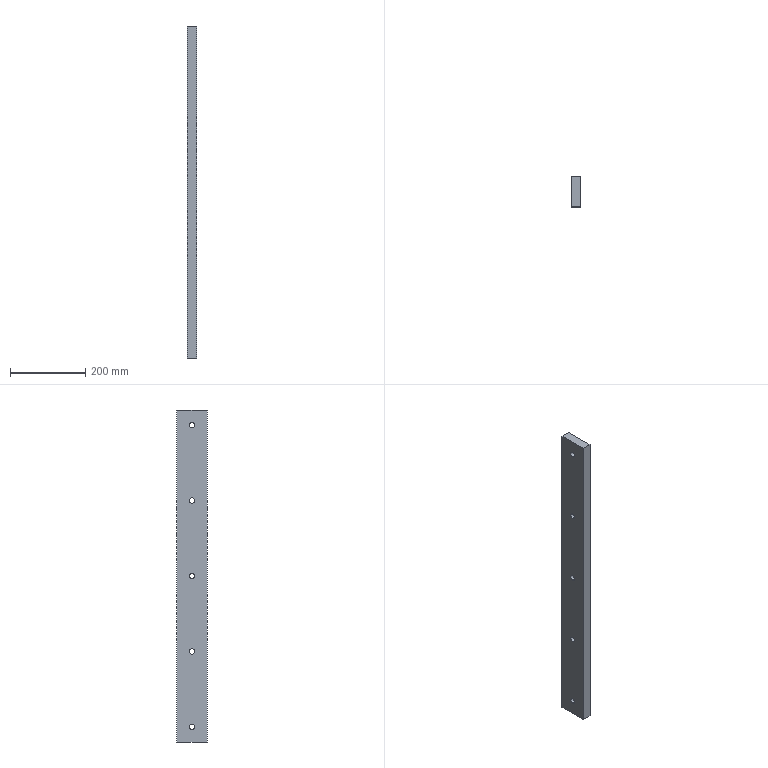Part | SolidWorks | features BaseBody 1 | 1 solid | 16 faces | box 25 x 80 x 880 mm | volume 1740758 mm3 | cylinder 10 | plane 6 | commonest cylinder face diameters 14 x10
STEP:
#1=CARTESIAN_POINT('',(-12.5,0.,407.));
#2=VERTEX_POINT('',#1);
#3=CARTESIAN_POINT('',(-12.5,0.,393.));
#4=VERTEX_POINT('',#3);
#5=CARTESIAN_POINT('',(-12.5,0.,400.));
#6=DIRECTION('',(1.,0.,0.));
#7=DIRECTION('',(0.,0.,-1.));
#8=AXIS2_PLACEMENT_3D('',#5,#6,#7);
#9=CIRCLE('',#8,7.);
#10=EDGE_CURVE('',#2,#4,#9,.T.);
#11=ORIENTED_EDGE('',*,*,#10,.F.);
#12=CARTESIAN_POINT('',(12.5,0.,407.));
#13=VERTEX_POINT('',#12);
#14=CARTESIAN_POINT('',(12.5,0.,407.));
#15=DIRECTION('',(1.,0.,0.));
#16=VECTOR('',#15,1000.);
#17=LINE('',#14,#16);
#18=EDGE_CURVE('',#2,#13,#17,.T.);
#19=ORIENTED_EDGE('',*,*,#18,.T.);
#20=CARTESIAN_POINT('',(12.5,0.,393.));
#21=VERTEX_POINT('',#20);
#22=CARTESIAN_POINT('',(12.5,0.,400.));
#23=DIRECTION('',(1.,0.,0.));
#24=DIRECTION('',(0.,0.,-1.));
#25=AXIS2_PLACEMENT_3D('',#22,#23,#24);
#26=CIRCLE('',#25,7.);
#27=EDGE_CURVE('',#13,#21,#26,.T.);
#28=ORIENTED_EDGE('',*,*,#27,.T.);
#29=CARTESIAN_POINT('',(12.5,0.,393.));
#30=DIRECTION('',(1.,0.,0.));
#31=VECTOR('',#30,1000.);
#32=LINE('',#29,#31);
#33=EDGE_CURVE('',#4,#21,#32,.T.);
#34=ORIENTED_EDGE('',*,*,#33,.F.);
#35=EDGE_LOOP('',(#11,#19,#28,#34));
#36=FACE_OUTER_BOUND('',#35,.T.);
#37=CARTESIAN_POINT('',(12.5,0.,400.));
#38=DIRECTION('',(1.,0.,0.));
#39=DIRECTION('',(0.,0.,-1.));
#40=AXIS2_PLACEMENT_3D('',#37,#38,#39);
#41=CYLINDRICAL_SURFACE('',#40,7.);
#42=ADVANCED_FACE('',(#36),#41,.F.);
#43=CARTESIAN_POINT('',(-12.5,0.,207.));
#44=VERTEX_POINT('',#43);
#45=CARTESIAN_POINT('',(-12.5,0.,193.));
#46=VERTEX_POINT('',#45);
#47=CARTESIAN_POINT('',(-12.5,0.,200.));
#48=DIRECTION('',(1.,0.,0.));
#49=DIRECTION('',(0.,0.,-1.));
#50=AXIS2_PLACEMENT_3D('',#47,#48,#49);
#51=CIRCLE('',#50,7.);
#52=EDGE_CURVE('',#44,#46,#51,.T.);
#53=ORIENTED_EDGE('',*,*,#52,.F.);
#54=CARTESIAN_POINT('',(12.5,0.,207.));
#55=VERTEX_POINT('',#54);
#56=CARTESIAN_POINT('',(12.5,0.,207.));
#57=DIRECTION('',(1.,0.,0.));
#58=VECTOR('',#57,1000.);
#59=LINE('',#56,#58);
#60=EDGE_CURVE('',#44,#55,#59,.T.);
#61=ORIENTED_EDGE('',*,*,#60,.T.);
#62=CARTESIAN_POINT('',(12.5,0.,193.));
#63=VERTEX_POINT('',#62);
#64=CARTESIAN_POINT('',(12.5,0.,200.));
#65=DIRECTION('',(1.,0.,0.));
#66=DIRECTION('',(0.,0.,-1.));
#67=AXIS2_PLACEMENT_3D('',#64,#65,#66);
#68=CIRCLE('',#67,7.);
#69=EDGE_CURVE('',#55,#63,#68,.T.);
#70=ORIENTED_EDGE('',*,*,#69,.T.);
#71=CARTESIAN_POINT('',(12.5,0.,193.));
#72=DIRECTION('',(1.,0.,0.));
#73=VECTOR('',#72,1000.);
#74=LINE('',#71,#73);
#75=EDGE_CURVE('',#46,#63,#74,.T.);
#76=ORIENTED_EDGE('',*,*,#75,.F.);
#77=EDGE_LOOP('',(#53,#61,#70,#76));
#78=FACE_OUTER_BOUND('',#77,.T.);
#79=CARTESIAN_POINT('',(12.5,0.,200.));
#80=DIRECTION('',(1.,0.,0.));
#81=DIRECTION('',(0.,0.,-1.));
#82=AXIS2_PLACEMENT_3D('',#79,#80,#81);
#83=CYLINDRICAL_SURFACE('',#82,7.);
#84=ADVANCED_FACE('',(#78),#83,.F.);
#85=CARTESIAN_POINT('',(-12.5,0.,7.));
#86=VERTEX_POINT('',#85);
#87=CARTESIAN_POINT('',(-12.5,0.,-7.));
#88=VERTEX_POINT('',#87);
#89=CARTESIAN_POINT('',(-12.5,0.,0.));
#90=DIRECTION('',(1.,0.,0.));
#91=DIRECTION('',(0.,0.,-1.));
#92=AXIS2_PLACEMENT_3D('',#89,#90,#91);
#93=CIRCLE('',#92,7.);
#94=EDGE_CURVE('',#86,#88,#93,.T.);
#95=ORIENTED_EDGE('',*,*,#94,.F.);
#96=CARTESIAN_POINT('',(12.5,0.,7.));
#97=VERTEX_POINT('',#96);
#98=CARTESIAN_POINT('',(12.5,0.,7.));
#99=DIRECTION('',(1.,0.,0.));
#100=VECTOR('',#99,1000.);
#101=LINE('',#98,#100);
#102=EDGE_CURVE('',#86,#97,#101,.T.);
#103=ORIENTED_EDGE('',*,*,#102,.T.);
#104=CARTESIAN_POINT('',(12.5,0.,-7.));
#105=VERTEX_POINT('',#104);
#106=CARTESIAN_POINT('',(12.5,0.,0.));
#107=DIRECTION('',(1.,0.,0.));
#108=DIRECTION('',(0.,0.,-1.));
#109=AXIS2_PLACEMENT_3D('',#106,#107,#108);
#110=CIRCLE('',#109,7.);
#111=EDGE_CURVE('',#97,#105,#110,.T.);
#112=ORIENTED_EDGE('',*,*,#111,.T.);
#113=CARTESIAN_POINT('',(12.5,0.,-7.));
#114=DIRECTION('',(1.,0.,0.));
#115=VECTOR('',#114,1000.);
#116=LINE('',#113,#115);
#117=EDGE_CURVE('',#88,#105,#116,.T.);
#118=ORIENTED_EDGE('',*,*,#117,.F.);
#119=EDGE_LOOP('',(#95,#103,#112,#118));
#120=FACE_OUTER_BOUND('',#119,.T.);
#121=CARTESIAN_POINT('',(12.5,0.,0.));
#122=DIRECTION('',(1.,0.,0.));
#123=DIRECTION('',(0.,0.,-1.));
#124=AXIS2_PLACEMENT_3D('',#121,#122,#123);
#125=CYLINDRICAL_SURFACE('',#124,7.);
#126=ADVANCED_FACE('',(#120),#125,.F.);
#127=CARTESIAN_POINT('',(-12.5,0.,-193.));
#128=VERTEX_POINT('',#127);
#129=CARTESIAN_POINT('',(-12.5,0.,-207.));
#130=VERTEX_POINT('',#129);
#131=CARTESIAN_POINT('',(-12.5,0.,-200.));
#132=DIRECTION('',(1.,0.,0.));
#133=DIRECTION('',(0.,0.,-1.));
#134=AXIS2_PLACEMENT_3D('',#131,#132,#133);
#135=CIRCLE('',#134,7.);
#136=EDGE_CURVE('',#128,#130,#135,.T.);
#137=ORIENTED_EDGE('',*,*,#136,.F.);
#138=CARTESIAN_POINT('',(12.5,0.,-193.));
#139=VERTEX_POINT('',#138);
#140=CARTESIAN_POINT('',(12.5,0.,-193.));
#141=DIRECTION('',(1.,0.,0.));
#142=VECTOR('',#141,1000.);
#143=LINE('',#140,#142);
#144=EDGE_CURVE('',#128,#139,#143,.T.);
#145=ORIENTED_EDGE('',*,*,#144,.T.);
#146=CARTESIAN_POINT('',(12.5,0.,-207.));
#147=VERTEX_POINT('',#146);
#148=CARTESIAN_POINT('',(12.5,0.,-200.));
#149=DIRECTION('',(1.,0.,0.));
#150=DIRECTION('',(0.,0.,-1.));
#151=AXIS2_PLACEMENT_3D('',#148,#149,#150);
#152=CIRCLE('',#151,7.);
#153=EDGE_CURVE('',#139,#147,#152,.T.);
#154=ORIENTED_EDGE('',*,*,#153,.T.);
#155=CARTESIAN_POINT('',(12.5,0.,-207.));
#156=DIRECTION('',(1.,0.,0.));
#157=VECTOR('',#156,1000.);
#158=LINE('',#155,#157);
#159=EDGE_CURVE('',#130,#147,#158,.T.);
#160=ORIENTED_EDGE('',*,*,#159,.F.);
#161=EDGE_LOOP('',(#137,#145,#154,#160));
#162=FACE_OUTER_BOUND('',#161,.T.);
#163=CARTESIAN_POINT('',(12.5,0.,-200.));
#164=DIRECTION('',(1.,0.,0.));
#165=DIRECTION('',(0.,0.,-1.));
#166=AXIS2_PLACEMENT_3D('',#163,#164,#165);
#167=CYLINDRICAL_SURFACE('',#166,7.);
#168=ADVANCED_FACE('',(#162),#167,.F.);
#169=CARTESIAN_POINT('',(-12.5,0.,-393.));
#170=VERTEX_POINT('',#169);
#171=CARTESIAN_POINT('',(-12.5,0.,-407.));
#172=VERTEX_POINT('',#171);
#173=CARTESIAN_POINT('',(-12.5,0.,-400.));
#174=DIRECTION('',(1.,0.,0.));
#175=DIRECTION('',(0.,0.,-1.));
#176=AXIS2_PLACEMENT_3D('',#173,#174,#175);
#177=CIRCLE('',#176,7.);
#178=EDGE_CURVE('',#170,#172,#177,.T.);
#179=ORIENTED_EDGE('',*,*,#178,.F.);
#180=CARTESIAN_POINT('',(12.5,0.,-393.));
#181=VERTEX_POINT('',#180);
#182=CARTESIAN_POINT('',(12.5,0.,-393.));
#183=DIRECTION('',(1.,0.,0.));
#184=VECTOR('',#183,1000.);
#185=LINE('',#182,#184);
#186=EDGE_CURVE('',#170,#181,#185,.T.);
#187=ORIENTED_EDGE('',*,*,#186,.T.);
#188=CARTESIAN_POINT('',(12.5,0.,-407.));
#189=VERTEX_POINT('',#188);
#190=CARTESIAN_POINT('',(12.5,0.,-400.));
#191=DIRECTION('',(1.,0.,0.));
#192=DIRECTION('',(0.,0.,-1.));
#193=AXIS2_PLACEMENT_3D('',#190,#191,#192);
#194=CIRCLE('',#193,7.);
#195=EDGE_CURVE('',#181,#189,#194,.T.);
#196=ORIENTED_EDGE('',*,*,#195,.T.);
#197=CARTESIAN_POINT('',(12.5,0.,-407.));
#198=DIRECTION('',(1.,0.,0.));
#199=VECTOR('',#198,1000.);
#200=LINE('',#197,#199);
#201=EDGE_CURVE('',#172,#189,#200,.T.);
#202=ORIENTED_EDGE('',*,*,#201,.F.);
#203=EDGE_LOOP('',(#179,#187,#196,#202));
#204=FACE_OUTER_BOUND('',#203,.T.);
#205=CARTESIAN_POINT('',(12.5,0.,-400.));
#206=DIRECTION('',(1.,0.,0.));
#207=DIRECTION('',(0.,0.,-1.));
#208=AXIS2_PLACEMENT_3D('',#205,#206,#207);
#209=CYLINDRICAL_SURFACE('',#208,7.);
#210=ADVANCED_FACE('',(#204),#209,.F.);
#211=CARTESIAN_POINT('',(-12.5,-40.,-440.));
#212=VERTEX_POINT('',#211);
#213=CARTESIAN_POINT('',(-12.5,40.,-440.));
#214=VERTEX_POINT('',#213);
#215=CARTESIAN_POINT('',(-12.5,40.,-440.));
#216=DIRECTION('',(0.,1.,0.));
#217=VECTOR('',#216,1000.);
#218=LINE('',#215,#217);
#219=EDGE_CURVE('',#212,#214,#218,.T.);
#220=ORIENTED_EDGE('',*,*,#219,.T.);
#221=CARTESIAN_POINT('',(12.5,40.,-440.));
#222=VERTEX_POINT('',#221);
#223=CARTESIAN_POINT('',(12.5,40.,-440.));
#224=DIRECTION('',(-1.,0.,0.));
#225=VECTOR('',#224,1000.);
#226=LINE('',#223,#225);
#227=EDGE_CURVE('',#222,#214,#226,.T.);
#228=ORIENTED_EDGE('',*,*,#227,.F.);
#229=CARTESIAN_POINT('',(12.5,-40.,-440.));
#230=VERTEX_POINT('',#229);
#231=CARTESIAN_POINT('',(12.5,40.,-440.));
#232=DIRECTION('',(0.,1.,0.));
#233=VECTOR('',#232,1000.);
#234=LINE('',#231,#233);
#235=EDGE_CURVE('',#230,#222,#234,.T.);
#236=ORIENTED_EDGE('',*,*,#235,.F.);
#237=CARTESIAN_POINT('',(12.5,-40.,-440.));
#238=DIRECTION('',(-1.,0.,0.));
#239=VECTOR('',#238,1000.);
#240=LINE('',#237,#239);
#241=EDGE_CURVE('',#230,#212,#240,.T.);
#242=ORIENTED_EDGE('',*,*,#241,.T.);
#243=EDGE_LOOP('',(#220,#228,#236,#242));
#244=FACE_OUTER_BOUND('',#243,.T.);
#245=CARTESIAN_POINT('',(12.5,40.,-440.));
#246=DIRECTION('',(0.,0.,1.));
#247=DIRECTION('',(1.,0.,0.));
#248=AXIS2_PLACEMENT_3D('',#245,#246,#247);
#249=PLANE('',#248);
#250=ADVANCED_FACE('',(#244),#249,.F.);
#251=CARTESIAN_POINT('',(-12.5,40.,440.));
#252=VERTEX_POINT('',#251);
#253=CARTESIAN_POINT('',(-12.5,40.,440.));
#254=DIRECTION('',(0.,0.,1.));
#255=VECTOR('',#254,1000.);
#256=LINE('',#253,#255);
#257=EDGE_CURVE('',#214,#252,#256,.T.);
#258=ORIENTED_EDGE('',*,*,#257,.T.);
#259=CARTESIAN_POINT('',(12.5,40.,440.));
#260=VERTEX_POINT('',#259);
#261=CARTESIAN_POINT('',(12.5,40.,440.));
#262=DIRECTION('',(-1.,0.,0.));
#263=VECTOR('',#262,1000.);
#264=LINE('',#261,#263);
#265=EDGE_CURVE('',#260,#252,#264,.T.);
#266=ORIENTED_EDGE('',*,*,#265,.F.);
#267=CARTESIAN_POINT('',(12.5,40.,440.));
#268=DIRECTION('',(0.,0.,1.));
#269=VECTOR('',#268,1000.);
#270=LINE('',#267,#269);
#271=EDGE_CURVE('',#222,#260,#270,.T.);
#272=ORIENTED_EDGE('',*,*,#271,.F.);
#273=ORIENTED_EDGE('',*,*,#227,.T.);
#274=EDGE_LOOP('',(#258,#266,#272,#273));
#275=FACE_OUTER_BOUND('',#274,.T.);
#276=CARTESIAN_POINT('',(12.5,40.,440.));
#277=DIRECTION('',(0.,-1.,0.));
#278=DIRECTION('',(0.,0.,-1.));
#279=AXIS2_PLACEMENT_3D('',#276,#277,#278);
#280=PLANE('',#279);
#281=ADVANCED_FACE('',(#275),#280,.F.);
#282=CARTESIAN_POINT('',(-12.5,-40.,440.));
#283=VERTEX_POINT('',#282);
#284=CARTESIAN_POINT('',(-12.5,40.,440.));
#285=DIRECTION('',(0.,-1.,0.));
#286=VECTOR('',#285,1000.);
#287=LINE('',#284,#286);
#288=EDGE_CURVE('',#252,#283,#287,.T.);
#289=ORIENTED_EDGE('',*,*,#288,.T.);
#290=CARTESIAN_POINT('',(12.5,-40.,440.));
#291=VERTEX_POINT('',#290);
#292=CARTESIAN_POINT('',(12.5,-40.,440.));
#293=DIRECTION('',(-1.,0.,0.));
#294=VECTOR('',#293,1000.);
#295=LINE('',#292,#294);
#296=EDGE_CURVE('',#291,#283,#295,.T.);
#297=ORIENTED_EDGE('',*,*,#296,.F.);
#298=CARTESIAN_POINT('',(12.5,40.,440.));
#299=DIRECTION('',(0.,-1.,0.));
#300=VECTOR('',#299,1000.);
#301=LINE('',#298,#300);
#302=EDGE_CURVE('',#260,#291,#301,.T.);
#303=ORIENTED_EDGE('',*,*,#302,.F.);
#304=ORIENTED_EDGE('',*,*,#265,.T.);
#305=EDGE_LOOP('',(#289,#297,#303,#304));
#306=FACE_OUTER_BOUND('',#305,.T.);
#307=CARTESIAN_POINT('',(12.5,40.,440.));
#308=DIRECTION('',(0.,0.,-1.));
#309=DIRECTION('',(-1.,0.,0.));
#310=AXIS2_PLACEMENT_3D('',#307,#308,#309);
#311=PLANE('',#310);
#312=ADVANCED_FACE('',(#306),#311,.F.);
#313=CARTESIAN_POINT('',(-12.5,-40.,440.));
#314=DIRECTION('',(0.,0.,-1.));
#315=VECTOR('',#314,1000.);
#316=LINE('',#313,#315);
#317=EDGE_CURVE('',#283,#212,#316,.T.);
#318=ORIENTED_EDGE('',*,*,#317,.T.);
#319=ORIENTED_EDGE('',*,*,#241,.F.);
#320=CARTESIAN_POINT('',(12.5,-40.,440.));
#321=DIRECTION('',(0.,0.,-1.));
#322=VECTOR('',#321,1000.);
#323=LINE('',#320,#322);
#324=EDGE_CURVE('',#291,#230,#323,.T.);
#325=ORIENTED_EDGE('',*,*,#324,.F.);
#326=ORIENTED_EDGE('',*,*,#296,.T.);
#327=EDGE_LOOP('',(#318,#319,#325,#326));
#328=FACE_OUTER_BOUND('',#327,.T.);
#329=CARTESIAN_POINT('',(12.5,-40.,440.));
#330=DIRECTION('',(0.,1.,0.));
#331=DIRECTION('',(0.,0.,1.));
#332=AXIS2_PLACEMENT_3D('',#329,#330,#331);
#333=PLANE('',#332);
#334=ADVANCED_FACE('',(#328),#333,.F.);
#335=CARTESIAN_POINT('',(12.5,0.,400.));
#336=DIRECTION('',(1.,0.,0.));
#337=DIRECTION('',(0.,0.,-1.));
#338=AXIS2_PLACEMENT_3D('',#335,#336,#337);
#339=CIRCLE('',#338,7.);
#340=EDGE_CURVE('',#21,#13,#339,.T.);
#341=ORIENTED_EDGE('',*,*,#340,.F.);
#342=ORIENTED_EDGE('',*,*,#27,.F.);
#343=EDGE_LOOP('',(#341,#342));
#344=FACE_BOUND('',#343,.T.);
#345=CARTESIAN_POINT('',(12.5,0.,200.));
#346=DIRECTION('',(1.,0.,0.));
#347=DIRECTION('',(0.,0.,-1.));
#348=AXIS2_PLACEMENT_3D('',#345,#346,#347);
#349=CIRCLE('',#348,7.);
#350=EDGE_CURVE('',#63,#55,#349,.T.);
#351=ORIENTED_EDGE('',*,*,#350,.F.);
#352=ORIENTED_EDGE('',*,*,#69,.F.);
#353=EDGE_LOOP('',(#351,#352));
#354=FACE_BOUND('',#353,.T.);
#355=CARTESIAN_POINT('',(12.5,0.,0.));
#356=DIRECTION('',(1.,0.,0.));
#357=DIRECTION('',(0.,0.,-1.));
#358=AXIS2_PLACEMENT_3D('',#355,#356,#357);
#359=CIRCLE('',#358,7.);
#360=EDGE_CURVE('',#105,#97,#359,.T.);
#361=ORIENTED_EDGE('',*,*,#360,.F.);
#362=ORIENTED_EDGE('',*,*,#111,.F.);
#363=EDGE_LOOP('',(#361,#362));
#364=FACE_BOUND('',#363,.T.);
#365=CARTESIAN_POINT('',(12.5,0.,-200.));
#366=DIRECTION('',(1.,0.,0.));
#367=DIRECTION('',(0.,0.,-1.));
#368=AXIS2_PLACEMENT_3D('',#365,#366,#367);
#369=CIRCLE('',#368,7.);
#370=EDGE_CURVE('',#147,#139,#369,.T.);
#371=ORIENTED_EDGE('',*,*,#370,.F.);
#372=ORIENTED_EDGE('',*,*,#153,.F.);
#373=EDGE_LOOP('',(#371,#372));
#374=FACE_BOUND('',#373,.T.);
#375=CARTESIAN_POINT('',(12.5,0.,-400.));
#376=DIRECTION('',(1.,0.,0.));
#377=DIRECTION('',(0.,0.,-1.));
#378=AXIS2_PLACEMENT_3D('',#375,#376,#377);
#379=CIRCLE('',#378,7.);
#380=EDGE_CURVE('',#189,#181,#379,.T.);
#381=ORIENTED_EDGE('',*,*,#380,.F.);
#382=ORIENTED_EDGE('',*,*,#195,.F.);
#383=EDGE_LOOP('',(#381,#382));
#384=FACE_BOUND('',#383,.T.);
#385=ORIENTED_EDGE('',*,*,#235,.T.);
#386=ORIENTED_EDGE('',*,*,#271,.T.);
#387=ORIENTED_EDGE('',*,*,#302,.T.);
#388=ORIENTED_EDGE('',*,*,#324,.T.);
#389=EDGE_LOOP('',(#385,#386,#387,#388));
#390=FACE_OUTER_BOUND('',#389,.T.);
#391=CARTESIAN_POINT('',(12.5,0.,0.));
#392=DIRECTION('',(1.,0.,0.));
#393=DIRECTION('',(0.,0.,-1.));
#394=AXIS2_PLACEMENT_3D('',#391,#392,#393);
#395=PLANE('',#394);
#396=ADVANCED_FACE('',(#344,#354,#364,#374,#384,#390),#395,.T.);
#397=CARTESIAN_POINT('',(-12.5,0.,400.));
#398=DIRECTION('',(1.,0.,0.));
#399=DIRECTION('',(0.,0.,-1.));
#400=AXIS2_PLACEMENT_3D('',#397,#398,#399);
#401=CIRCLE('',#400,7.);
#402=EDGE_CURVE('',#4,#2,#401,.T.);
#403=ORIENTED_EDGE('',*,*,#402,.T.);
#404=ORIENTED_EDGE('',*,*,#10,.T.);
#405=EDGE_LOOP('',(#403,#404));
#406=FACE_BOUND('',#405,.T.);
#407=CARTESIAN_POINT('',(-12.5,0.,200.));
#408=DIRECTION('',(1.,0.,0.));
#409=DIRECTION('',(0.,0.,-1.));
#410=AXIS2_PLACEMENT_3D('',#407,#408,#409);
#411=CIRCLE('',#410,7.);
#412=EDGE_CURVE('',#46,#44,#411,.T.);
#413=ORIENTED_EDGE('',*,*,#412,.T.);
#414=ORIENTED_EDGE('',*,*,#52,.T.);
#415=EDGE_LOOP('',(#413,#414));
#416=FACE_BOUND('',#415,.T.);
#417=CARTESIAN_POINT('',(-12.5,0.,0.));
#418=DIRECTION('',(1.,0.,0.));
#419=DIRECTION('',(0.,0.,-1.));
#420=AXIS2_PLACEMENT_3D('',#417,#418,#419);
#421=CIRCLE('',#420,7.);
#422=EDGE_CURVE('',#88,#86,#421,.T.);
#423=ORIENTED_EDGE('',*,*,#422,.T.);
#424=ORIENTED_EDGE('',*,*,#94,.T.);
#425=EDGE_LOOP('',(#423,#424));
#426=FACE_BOUND('',#425,.T.);
#427=CARTESIAN_POINT('',(-12.5,0.,-200.));
#428=DIRECTION('',(1.,0.,0.));
#429=DIRECTION('',(0.,0.,-1.));
#430=AXIS2_PLACEMENT_3D('',#427,#428,#429);
#431=CIRCLE('',#430,7.);
#432=EDGE_CURVE('',#130,#128,#431,.T.);
#433=ORIENTED_EDGE('',*,*,#432,.T.);
#434=ORIENTED_EDGE('',*,*,#136,.T.);
#435=EDGE_LOOP('',(#433,#434));
#436=FACE_BOUND('',#435,.T.);
#437=CARTESIAN_POINT('',(-12.5,0.,-400.));
#438=DIRECTION('',(1.,0.,0.));
#439=DIRECTION('',(0.,0.,-1.));
#440=AXIS2_PLACEMENT_3D('',#437,#438,#439);
#441=CIRCLE('',#440,7.);
#442=EDGE_CURVE('',#172,#170,#441,.T.);
#443=ORIENTED_EDGE('',*,*,#442,.T.);
#444=ORIENTED_EDGE('',*,*,#178,.T.);
#445=EDGE_LOOP('',(#443,#444));
#446=FACE_BOUND('',#445,.T.);
#447=ORIENTED_EDGE('',*,*,#219,.F.);
#448=ORIENTED_EDGE('',*,*,#317,.F.);
#449=ORIENTED_EDGE('',*,*,#288,.F.);
#450=ORIENTED_EDGE('',*,*,#257,.F.);
#451=EDGE_LOOP('',(#447,#448,#449,#450));
#452=FACE_OUTER_BOUND('',#451,.T.);
#453=CARTESIAN_POINT('',(-12.5,0.,0.));
#454=DIRECTION('',(1.,0.,0.));
#455=DIRECTION('',(0.,0.,-1.));
#456=AXIS2_PLACEMENT_3D('',#453,#454,#455);
#457=PLANE('',#456);
#458=ADVANCED_FACE('',(#406,#416,#426,#436,#446,#452),#457,.F.);
#459=ORIENTED_EDGE('',*,*,#186,.F.);
#460=ORIENTED_EDGE('',*,*,#442,.F.);
#461=ORIENTED_EDGE('',*,*,#201,.T.);
#462=ORIENTED_EDGE('',*,*,#380,.T.);
#463=EDGE_LOOP('',(#459,#460,#461,#462));
#464=FACE_OUTER_BOUND('',#463,.T.);
#465=CARTESIAN_POINT('',(12.5,0.,-400.));
#466=DIRECTION('',(1.,0.,0.));
#467=DIRECTION('',(0.,0.,-1.));
#468=AXIS2_PLACEMENT_3D('',#465,#466,#467);
#469=CYLINDRICAL_SURFACE('',#468,7.);
#470=ADVANCED_FACE('',(#464),#469,.F.);
#471=ORIENTED_EDGE('',*,*,#144,.F.);
#472=ORIENTED_EDGE('',*,*,#432,.F.);
#473=ORIENTED_EDGE('',*,*,#159,.T.);
#474=ORIENTED_EDGE('',*,*,#370,.T.);
#475=EDGE_LOOP('',(#471,#472,#473,#474));
#476=FACE_OUTER_BOUND('',#475,.T.);
#477=CARTESIAN_POINT('',(12.5,0.,-200.));
#478=DIRECTION('',(1.,0.,0.));
#479=DIRECTION('',(0.,0.,-1.));
#480=AXIS2_PLACEMENT_3D('',#477,#478,#479);
#481=CYLINDRICAL_SURFACE('',#480,7.);
#482=ADVANCED_FACE('',(#476),#481,.F.);
#483=ORIENTED_EDGE('',*,*,#102,.F.);
#484=ORIENTED_EDGE('',*,*,#422,.F.);
#485=ORIENTED_EDGE('',*,*,#117,.T.);
#486=ORIENTED_EDGE('',*,*,#360,.T.);
#487=EDGE_LOOP('',(#483,#484,#485,#486));
#488=FACE_OUTER_BOUND('',#487,.T.);
#489=CARTESIAN_POINT('',(12.5,0.,0.));
#490=DIRECTION('',(1.,0.,0.));
#491=DIRECTION('',(0.,0.,-1.));
#492=AXIS2_PLACEMENT_3D('',#489,#490,#491);
#493=CYLINDRICAL_SURFACE('',#492,7.);
#494=ADVANCED_FACE('',(#488),#493,.F.);
#495=ORIENTED_EDGE('',*,*,#60,.F.);
#496=ORIENTED_EDGE('',*,*,#412,.F.);
#497=ORIENTED_EDGE('',*,*,#75,.T.);
#498=ORIENTED_EDGE('',*,*,#350,.T.);
#499=EDGE_LOOP('',(#495,#496,#497,#498));
#500=FACE_OUTER_BOUND('',#499,.T.);
#501=CARTESIAN_POINT('',(12.5,0.,200.));
#502=DIRECTION('',(1.,0.,0.));
#503=DIRECTION('',(0.,0.,-1.));
#504=AXIS2_PLACEMENT_3D('',#501,#502,#503);
#505=CYLINDRICAL_SURFACE('',#504,7.);
#506=ADVANCED_FACE('',(#500),#505,.F.);
#507=ORIENTED_EDGE('',*,*,#18,.F.);
#508=ORIENTED_EDGE('',*,*,#402,.F.);
#509=ORIENTED_EDGE('',*,*,#33,.T.);
#510=ORIENTED_EDGE('',*,*,#340,.T.);
#511=EDGE_LOOP('',(#507,#508,#509,#510));
#512=FACE_OUTER_BOUND('',#511,.T.);
#513=CARTESIAN_POINT('',(12.5,0.,400.));
#514=DIRECTION('',(1.,0.,0.));
#515=DIRECTION('',(0.,0.,-1.));
#516=AXIS2_PLACEMENT_3D('',#513,#514,#515);
#517=CYLINDRICAL_SURFACE('',#516,7.);
#518=ADVANCED_FACE('',(#512),#517,.F.);
#519=CLOSED_SHELL('',(#42,#84,#126,#168,#210,#250,#281,#312,#334,#396,#458,#470,#482,#494,#506,#518));
#520=MANIFOLD_SOLID_BREP('',#519);
#521=CARTESIAN_POINT('',(0.,0.,0.));
#522=DIRECTION('',(0.,0.,1.));
#523=DIRECTION('',(1.,0.,0.));
#524=AXIS2_PLACEMENT_3D('',#521,#522,#523);
#525=(LENGTH_UNIT()NAMED_UNIT(*)SI_UNIT(.MILLI.,.METRE.));
#526=UNCERTAINTY_MEASURE_WITH_UNIT(LENGTH_MEASURE(0.00001),#525,'','');
#527=(NAMED_UNIT(*)PLANE_ANGLE_UNIT()SI_UNIT($,.RADIAN.));
#528=(NAMED_UNIT(*)SI_UNIT($,.STERADIAN.)SOLID_ANGLE_UNIT());
#529=(GEOMETRIC_REPRESENTATION_CONTEXT(3)GLOBAL_UNCERTAINTY_ASSIGNED_CONTEXT((#526))GLOBAL_UNIT_ASSIGNED_CONTEXT((#525,#527,#528))REPRESENTATION_CONTEXT('',''));
#530=ADVANCED_BREP_SHAPE_REPRESENTATION('',(#520,#524),#529);